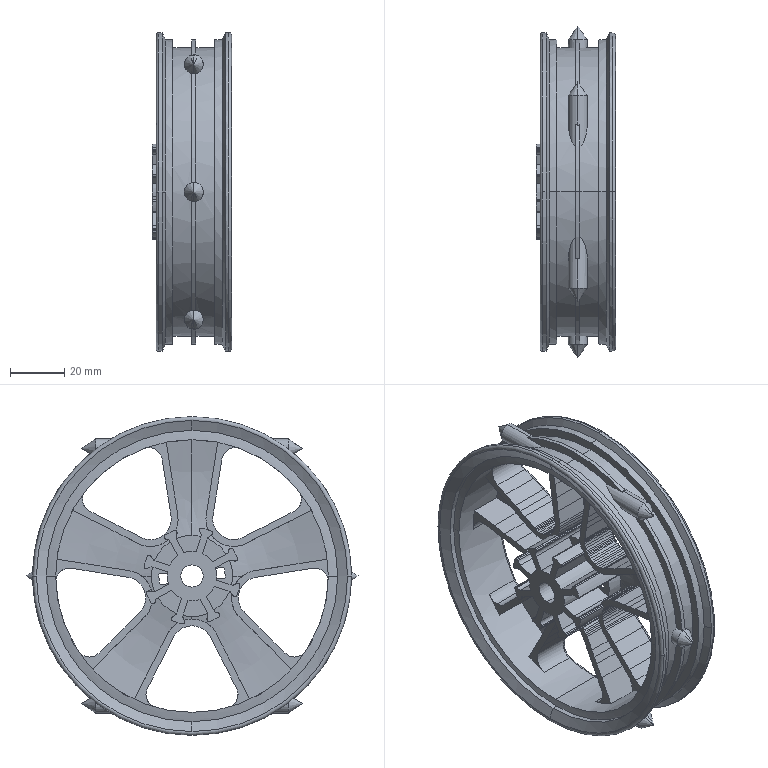Part | SolidWorks | features BaseBody 1, ICE 1 | 1 solid | 698 faces | box 29.19 x 122.462 x 117.58 mm | volume 68674 mm3 | spline 450 | cylinder 135 | plane 65 | torus 28 | cone 20 | commonest cylinder face diameters 1 x38 4 x18 7 x12 10 x12 112.462 x11 18.2 x9